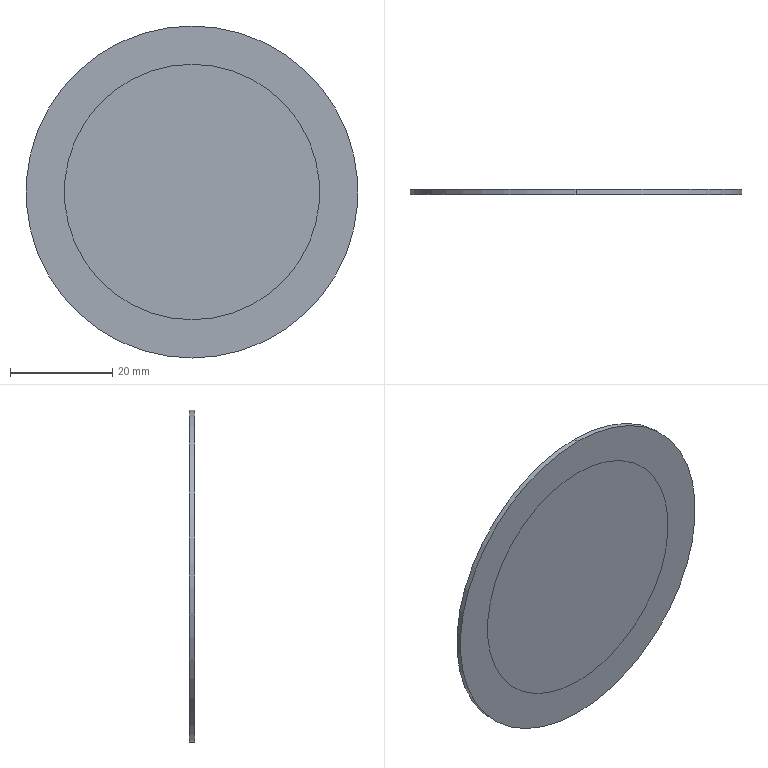Part | SolidWorks | features Extrusion 1, ICE 1 | 2 solids | 10 faces | box 65 x 1 x 65 mm | volume 3318 mm3 | cylinder 6 | plane 4 | commonest cylinder face diameters 50 x4 65 x2
STEP:
#1=CARTESIAN_POINT('',(0.,1.,-25.));
#2=VERTEX_POINT('',#1);
#3=CARTESIAN_POINT('',(0.,1.,25.));
#4=VERTEX_POINT('',#3);
#5=CARTESIAN_POINT('',(0.,1.,0.));
#6=DIRECTION('',(0.,1.,0.));
#7=DIRECTION('',(0.,0.,1.));
#8=AXIS2_PLACEMENT_3D('',#5,#6,#7);
#9=CIRCLE('',#8,25.);
#10=EDGE_CURVE('',#2,#4,#9,.T.);
#11=ORIENTED_EDGE('',*,*,#10,.T.);
#12=CARTESIAN_POINT('',(0.,0.,25.));
#13=VERTEX_POINT('',#12);
#14=CARTESIAN_POINT('',(0.,1.,25.));
#15=DIRECTION('',(0.,-1.,0.));
#16=VECTOR('',#15,1000.);
#17=LINE('',#14,#16);
#18=EDGE_CURVE('',#4,#13,#17,.T.);
#19=ORIENTED_EDGE('',*,*,#18,.T.);
#20=CARTESIAN_POINT('',(0.,0.,-25.));
#21=VERTEX_POINT('',#20);
#22=CARTESIAN_POINT('',(0.,0.,0.));
#23=DIRECTION('',(0.,1.,0.));
#24=DIRECTION('',(0.,0.,1.));
#25=AXIS2_PLACEMENT_3D('',#22,#23,#24);
#26=CIRCLE('',#25,25.);
#27=EDGE_CURVE('',#21,#13,#26,.T.);
#28=ORIENTED_EDGE('',*,*,#27,.F.);
#29=CARTESIAN_POINT('',(0.,1.,-25.));
#30=DIRECTION('',(0.,-1.,0.));
#31=VECTOR('',#30,1000.);
#32=LINE('',#29,#31);
#33=EDGE_CURVE('',#2,#21,#32,.T.);
#34=ORIENTED_EDGE('',*,*,#33,.F.);
#35=EDGE_LOOP('',(#11,#19,#28,#34));
#36=FACE_OUTER_BOUND('',#35,.T.);
#37=CARTESIAN_POINT('',(0.,1.,0.));
#38=DIRECTION('',(0.,-1.,0.));
#39=DIRECTION('',(0.,0.,-1.));
#40=AXIS2_PLACEMENT_3D('',#37,#38,#39);
#41=CYLINDRICAL_SURFACE('',#40,25.);
#42=ADVANCED_FACE('',(#36),#41,.F.);
#43=CARTESIAN_POINT('',(0.,1.,32.5));
#44=VERTEX_POINT('',#43);
#45=CARTESIAN_POINT('',(0.,1.,-32.5));
#46=VERTEX_POINT('',#45);
#47=CARTESIAN_POINT('',(0.,1.,0.));
#48=DIRECTION('',(0.,1.,0.));
#49=DIRECTION('',(0.,0.,1.));
#50=AXIS2_PLACEMENT_3D('',#47,#48,#49);
#51=CIRCLE('',#50,32.5);
#52=EDGE_CURVE('',#44,#46,#51,.T.);
#53=ORIENTED_EDGE('',*,*,#52,.F.);
#54=CARTESIAN_POINT('',(0.,0.,32.5));
#55=VERTEX_POINT('',#54);
#56=CARTESIAN_POINT('',(0.,1.,32.5));
#57=DIRECTION('',(0.,-1.,0.));
#58=VECTOR('',#57,1000.);
#59=LINE('',#56,#58);
#60=EDGE_CURVE('',#44,#55,#59,.T.);
#61=ORIENTED_EDGE('',*,*,#60,.T.);
#62=CARTESIAN_POINT('',(0.,0.,-32.5));
#63=VERTEX_POINT('',#62);
#64=CARTESIAN_POINT('',(0.,0.,0.));
#65=DIRECTION('',(0.,1.,0.));
#66=DIRECTION('',(0.,0.,1.));
#67=AXIS2_PLACEMENT_3D('',#64,#65,#66);
#68=CIRCLE('',#67,32.5);
#69=EDGE_CURVE('',#55,#63,#68,.T.);
#70=ORIENTED_EDGE('',*,*,#69,.T.);
#71=CARTESIAN_POINT('',(0.,1.,-32.5));
#72=DIRECTION('',(0.,-1.,0.));
#73=VECTOR('',#72,1000.);
#74=LINE('',#71,#73);
#75=EDGE_CURVE('',#46,#63,#74,.T.);
#76=ORIENTED_EDGE('',*,*,#75,.F.);
#77=EDGE_LOOP('',(#53,#61,#70,#76));
#78=FACE_OUTER_BOUND('',#77,.T.);
#79=CARTESIAN_POINT('',(0.,1.,0.));
#80=DIRECTION('',(0.,-1.,0.));
#81=DIRECTION('',(0.,0.,-1.));
#82=AXIS2_PLACEMENT_3D('',#79,#80,#81);
#83=CYLINDRICAL_SURFACE('',#82,32.5);
#84=ADVANCED_FACE('',(#78),#83,.T.);
#85=CARTESIAN_POINT('',(0.,1.,0.));
#86=DIRECTION('',(0.,1.,0.));
#87=DIRECTION('',(0.,0.,1.));
#88=AXIS2_PLACEMENT_3D('',#85,#86,#87);
#89=CIRCLE('',#88,32.5);
#90=EDGE_CURVE('',#46,#44,#89,.T.);
#91=ORIENTED_EDGE('',*,*,#90,.T.);
#92=ORIENTED_EDGE('',*,*,#52,.T.);
#93=EDGE_LOOP('',(#91,#92));
#94=FACE_OUTER_BOUND('',#93,.T.);
#95=ORIENTED_EDGE('',*,*,#10,.F.);
#96=CARTESIAN_POINT('',(0.,1.,0.));
#97=DIRECTION('',(0.,1.,0.));
#98=DIRECTION('',(0.,0.,1.));
#99=AXIS2_PLACEMENT_3D('',#96,#97,#98);
#100=CIRCLE('',#99,25.);
#101=EDGE_CURVE('',#4,#2,#100,.T.);
#102=ORIENTED_EDGE('',*,*,#101,.F.);
#103=EDGE_LOOP('',(#95,#102));
#104=FACE_BOUND('',#103,.T.);
#105=CARTESIAN_POINT('',(0.,1.,0.));
#106=DIRECTION('',(0.,1.,0.));
#107=DIRECTION('',(0.,0.,1.));
#108=AXIS2_PLACEMENT_3D('',#105,#106,#107);
#109=PLANE('',#108);
#110=ADVANCED_FACE('',(#94,#104),#109,.T.);
#111=CARTESIAN_POINT('',(0.,0.,0.));
#112=DIRECTION('',(0.,1.,0.));
#113=DIRECTION('',(0.,0.,1.));
#114=AXIS2_PLACEMENT_3D('',#111,#112,#113);
#115=CIRCLE('',#114,32.5);
#116=EDGE_CURVE('',#63,#55,#115,.T.);
#117=ORIENTED_EDGE('',*,*,#116,.F.);
#118=ORIENTED_EDGE('',*,*,#69,.F.);
#119=EDGE_LOOP('',(#117,#118));
#120=FACE_OUTER_BOUND('',#119,.T.);
#121=ORIENTED_EDGE('',*,*,#27,.T.);
#122=CARTESIAN_POINT('',(0.,0.,0.));
#123=DIRECTION('',(0.,1.,0.));
#124=DIRECTION('',(0.,0.,1.));
#125=AXIS2_PLACEMENT_3D('',#122,#123,#124);
#126=CIRCLE('',#125,25.);
#127=EDGE_CURVE('',#13,#21,#126,.T.);
#128=ORIENTED_EDGE('',*,*,#127,.T.);
#129=EDGE_LOOP('',(#121,#128));
#130=FACE_BOUND('',#129,.T.);
#131=CARTESIAN_POINT('',(0.,0.,0.));
#132=DIRECTION('',(0.,1.,0.));
#133=DIRECTION('',(0.,0.,1.));
#134=AXIS2_PLACEMENT_3D('',#131,#132,#133);
#135=PLANE('',#134);
#136=ADVANCED_FACE('',(#120,#130),#135,.F.);
#137=ORIENTED_EDGE('',*,*,#60,.F.);
#138=ORIENTED_EDGE('',*,*,#90,.F.);
#139=ORIENTED_EDGE('',*,*,#75,.T.);
#140=ORIENTED_EDGE('',*,*,#116,.T.);
#141=EDGE_LOOP('',(#137,#138,#139,#140));
#142=FACE_OUTER_BOUND('',#141,.T.);
#143=CARTESIAN_POINT('',(0.,1.,0.));
#144=DIRECTION('',(0.,-1.,0.));
#145=DIRECTION('',(0.,0.,-1.));
#146=AXIS2_PLACEMENT_3D('',#143,#144,#145);
#147=CYLINDRICAL_SURFACE('',#146,32.5);
#148=ADVANCED_FACE('',(#142),#147,.T.);
#149=ORIENTED_EDGE('',*,*,#18,.F.);
#150=ORIENTED_EDGE('',*,*,#101,.T.);
#151=ORIENTED_EDGE('',*,*,#33,.T.);
#152=ORIENTED_EDGE('',*,*,#127,.F.);
#153=EDGE_LOOP('',(#149,#150,#151,#152));
#154=FACE_OUTER_BOUND('',#153,.T.);
#155=CARTESIAN_POINT('',(0.,1.,0.));
#156=DIRECTION('',(0.,-1.,0.));
#157=DIRECTION('',(0.,0.,-1.));
#158=AXIS2_PLACEMENT_3D('',#155,#156,#157);
#159=CYLINDRICAL_SURFACE('',#158,25.);
#160=ADVANCED_FACE('',(#154),#159,.F.);
#161=CLOSED_SHELL('',(#42,#84,#110,#136,#148,#160));
#162=MANIFOLD_SOLID_BREP('',#161);
#163=CARTESIAN_POINT('',(0.,1.,-25.));
#164=VERTEX_POINT('',#163);
#165=CARTESIAN_POINT('',(0.,1.,25.));
#166=VERTEX_POINT('',#165);
#167=CARTESIAN_POINT('',(0.,1.,0.));
#168=DIRECTION('',(0.,-1.,0.));
#169=DIRECTION('',(0.,0.,1.));
#170=AXIS2_PLACEMENT_3D('',#167,#168,#169);
#171=CIRCLE('',#170,25.);
#172=EDGE_CURVE('',#164,#166,#171,.T.);
#173=ORIENTED_EDGE('',*,*,#172,.T.);
#174=CARTESIAN_POINT('',(0.,0.,25.));
#175=VERTEX_POINT('',#174);
#176=CARTESIAN_POINT('',(0.,71.711,25.));
#177=DIRECTION('',(0.,-1.,0.));
#178=VECTOR('',#177,1000.);
#179=LINE('',#176,#178);
#180=EDGE_CURVE('',#166,#175,#179,.T.);
#181=ORIENTED_EDGE('',*,*,#180,.T.);
#182=CARTESIAN_POINT('',(0.,0.,-25.));
#183=VERTEX_POINT('',#182);
#184=CARTESIAN_POINT('',(0.,0.,0.));
#185=DIRECTION('',(0.,-1.,0.));
#186=DIRECTION('',(0.,0.,-1.));
#187=AXIS2_PLACEMENT_3D('',#184,#185,#186);
#188=CIRCLE('',#187,25.);
#189=EDGE_CURVE('',#183,#175,#188,.T.);
#190=ORIENTED_EDGE('',*,*,#189,.F.);
#191=CARTESIAN_POINT('',(0.,71.711,-25.));
#192=DIRECTION('',(0.,-1.,0.));
#193=VECTOR('',#192,1000.);
#194=LINE('',#191,#193);
#195=EDGE_CURVE('',#164,#183,#194,.T.);
#196=ORIENTED_EDGE('',*,*,#195,.F.);
#197=EDGE_LOOP('',(#173,#181,#190,#196));
#198=FACE_OUTER_BOUND('',#197,.T.);
#199=CARTESIAN_POINT('',(0.,71.711,0.));
#200=DIRECTION('',(0.,-1.,0.));
#201=DIRECTION('',(0.,0.,-1.));
#202=AXIS2_PLACEMENT_3D('',#199,#200,#201);
#203=CYLINDRICAL_SURFACE('',#202,25.);
#204=ADVANCED_FACE('',(#198),#203,.T.);
#205=ORIENTED_EDGE('',*,*,#172,.F.);
#206=CARTESIAN_POINT('',(0.,1.,0.));
#207=DIRECTION('',(0.,-1.,0.));
#208=DIRECTION('',(0.,0.,1.));
#209=AXIS2_PLACEMENT_3D('',#206,#207,#208);
#210=CIRCLE('',#209,25.);
#211=EDGE_CURVE('',#166,#164,#210,.T.);
#212=ORIENTED_EDGE('',*,*,#211,.F.);
#213=EDGE_LOOP('',(#205,#212));
#214=FACE_OUTER_BOUND('',#213,.T.);
#215=CARTESIAN_POINT('',(0.,1.,0.));
#216=DIRECTION('',(0.,1.,0.));
#217=DIRECTION('',(0.,0.,1.));
#218=AXIS2_PLACEMENT_3D('',#215,#216,#217);
#219=PLANE('',#218);
#220=ADVANCED_FACE('',(#214),#219,.T.);
#221=ORIENTED_EDGE('',*,*,#189,.T.);
#222=CARTESIAN_POINT('',(0.,0.,0.));
#223=DIRECTION('',(0.,-1.,0.));
#224=DIRECTION('',(0.,0.,-1.));
#225=AXIS2_PLACEMENT_3D('',#222,#223,#224);
#226=CIRCLE('',#225,25.);
#227=EDGE_CURVE('',#175,#183,#226,.T.);
#228=ORIENTED_EDGE('',*,*,#227,.T.);
#229=EDGE_LOOP('',(#221,#228));
#230=FACE_OUTER_BOUND('',#229,.T.);
#231=CARTESIAN_POINT('',(0.,0.,0.));
#232=DIRECTION('',(0.,-1.,0.));
#233=DIRECTION('',(0.,0.,-1.));
#234=AXIS2_PLACEMENT_3D('',#231,#232,#233);
#235=PLANE('',#234);
#236=ADVANCED_FACE('',(#230),#235,.T.);
#237=ORIENTED_EDGE('',*,*,#180,.F.);
#238=ORIENTED_EDGE('',*,*,#211,.T.);
#239=ORIENTED_EDGE('',*,*,#195,.T.);
#240=ORIENTED_EDGE('',*,*,#227,.F.);
#241=EDGE_LOOP('',(#237,#238,#239,#240));
#242=FACE_OUTER_BOUND('',#241,.T.);
#243=CARTESIAN_POINT('',(0.,71.711,0.));
#244=DIRECTION('',(0.,-1.,0.));
#245=DIRECTION('',(0.,0.,-1.));
#246=AXIS2_PLACEMENT_3D('',#243,#244,#245);
#247=CYLINDRICAL_SURFACE('',#246,25.);
#248=ADVANCED_FACE('',(#242),#247,.T.);
#249=CLOSED_SHELL('',(#204,#220,#236,#248));
#250=MANIFOLD_SOLID_BREP('',#249);
#251=CARTESIAN_POINT('',(0.,0.,0.));
#252=DIRECTION('',(0.,0.,1.));
#253=DIRECTION('',(1.,0.,0.));
#254=AXIS2_PLACEMENT_3D('',#251,#252,#253);
#255=(LENGTH_UNIT()NAMED_UNIT(*)SI_UNIT(.MILLI.,.METRE.));
#256=UNCERTAINTY_MEASURE_WITH_UNIT(LENGTH_MEASURE(0.00001),#255,'','');
#257=(NAMED_UNIT(*)PLANE_ANGLE_UNIT()SI_UNIT($,.RADIAN.));
#258=(NAMED_UNIT(*)SI_UNIT($,.STERADIAN.)SOLID_ANGLE_UNIT());
#259=(GEOMETRIC_REPRESENTATION_CONTEXT(3)GLOBAL_UNCERTAINTY_ASSIGNED_CONTEXT((#256))GLOBAL_UNIT_ASSIGNED_CONTEXT((#255,#257,#258))REPRESENTATION_CONTEXT('',''));
#260=ADVANCED_BREP_SHAPE_REPRESENTATION('',(#162,#250,#254),#259);